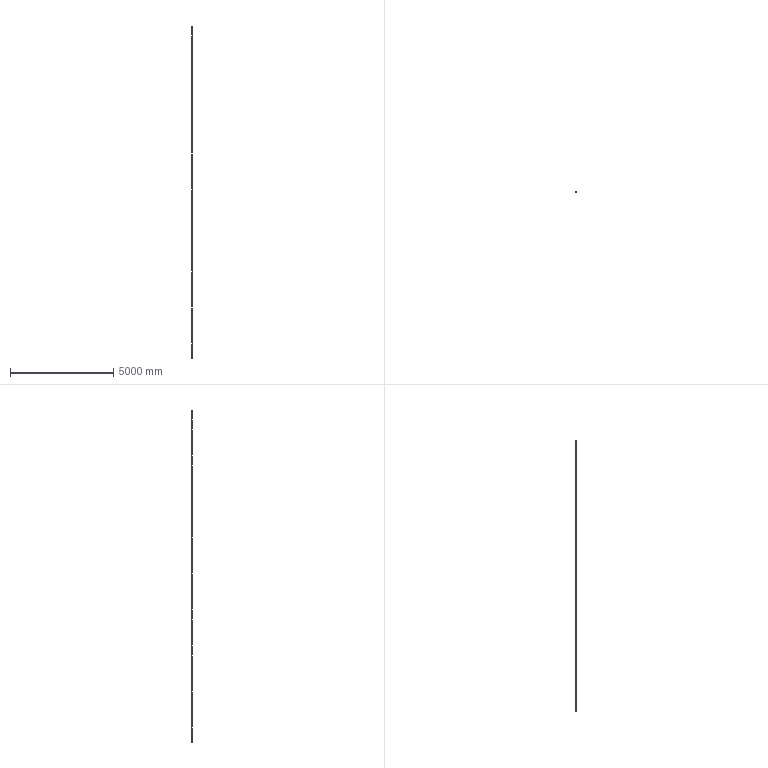Part | SolidWorks | features ICE 3, BaseBody 1, LPattern 1 | 1 solid | 1374 faces | box 23 x 22 x 16040 mm | volume 6693240 mm3 | cylinder 1076 | plane 298 | commonest cylinder face diameters 7 x536 11 x536 4.6 x4